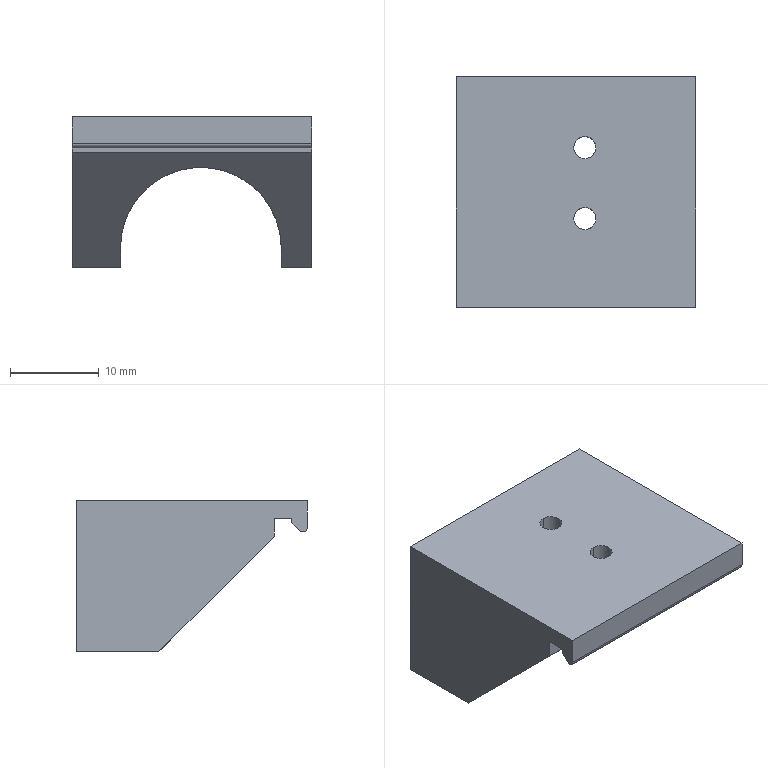NC program | NX | posted with a generic post | part box 27 x 26 x 17 mm
Lines 1 to 1768 of 22937, first 1687 of 1754 lines:
N10 G17 G21 G94 G90
(FLOOR_WALL , TOOL : D10JING)
N12 T09 M6
N14 G54
N16 G17 G0 G90 X-23.5 Y14.997 S9500 M3
N18 G43 Z30. H9
N20 Z3.
N22 G94 G1 Z0. F1250.
N24 X-20.5
N26 X20.5
N28 Y10.664
N30 X-20.5
N32 Y6.331
N34 X20.5
N36 Y1.999
N38 X-20.5
N40 Y-2.334
N42 X20.5
N44 Y-6.667
N46 X-20.5
N48 Y-11.
N50 X20.5
N52 X23.5
N54 Z3.
N56 G0 Z30.
N58 M5
(DRILLING , TOOL : D6A45)
N60 T07 M6
N62 G54
N64 G17 G0 G90 X-1. Y-3. S5000 M3
N66 G43 Z30. H7
N68 G94 G81 G98 Z-1. F250. R3.
N70 Y5.
N72 G80
N74 G0 X-1. Y5. Z30.
N76 M5
(DRILLING_COPY_COPY_COPY_COPY , TOOL : 2.5ZT)
N78 T08 M6
N80 G54
N82 G17 G0 G90 X-1. Y5. S2000 M3
N84 G43 Z30. H8
N86 G94 G83 G98 Z-19.251 F150. Q2. R3.
N88 Y-3.
N90 G80
N92 G0 X-1. Y-3. Z30.
N94 M5
(ZLEVEL_PROFILE , TOOL : D10)
N96 T10 M6
N98 G54
N100 G17 G0 G90 X16.359 Y-17.223 S9500 M3
N102 G43 Z30. H10
N104 Z1.5
N106 G94 G1 X15.398 Y-17.766 Z1.442 F1000.
N108 X14.054 Y-18.1 Z1.37
N110 X-14.054 Z-0.104
N112 X-15.398 Y-17.766 Z-0.176
N114 X-16.604 Y-17.084 Z-0.249
N116 X-17.584 Y-16.104 Z-0.321
N118 X-18.266 Y-14.898 Z-0.394
N120 X-18.6 Y-13.554 Z-0.467
N122 Y-13. Z-0.496
N124 Y13. F2500.
N126 G2 X-13.5 Y18.1 R5.1
N128 G1 X13.5
N130 G2 X18.6 Y13. R5.1
N132 G1 Y-13.
N134 G2 X13.5 Y-18.1 R5.1
N136 G1 X-13.5
N138 G2 X-18.6 Y-13. R5.1
N140 G1 Y12.323 Z-0.938
N142 Y12.706 Z-0.944
N144 X-18.599 Y13.09 Z-0.951
N146 X-18.578 Y13.473 Z-0.958
N148 X-18.528 Y13.853 Z-0.964
N150 X-18.45 Y14.229 Z-0.971
N152 X-18.343 Y14.598 Z-0.978
N154 X-18.21 Y14.957 Z-0.984
N156 X-18.049 Y15.305 Z-0.991
N158 G2 X-13.5 Y18.1 R5.1
N160 G1 X13.5
N162 G2 X18.6 Y13. R5.1
N164 G1 Y-13.
N166 G2 X13.5 Y-18.1 R5.1
N168 G1 X-13.5
N170 G2 X-18.6 Y-13. R5.1
N172 G1 Y12.323 Z-1.433
N174 Y12.706 Z-1.44
N176 X-18.599 Y13.09 Z-1.447
N178 X-18.578 Y13.473 Z-1.453
N180 X-18.528 Y13.853 Z-1.46
N182 X-18.45 Y14.229 Z-1.467
N184 X-18.343 Y14.598 Z-1.473
N186 X-18.21 Y14.957 Z-1.48
N188 X-18.049 Y15.305 Z-1.487
N190 G2 X-13.5 Y18.1 R5.1
N192 G1 X13.5
N194 G2 X18.6 Y13. R5.1
N196 G1 Y-13.
N198 G2 X13.5 Y-18.1 R5.1
N200 G1 X-13.5
N202 G2 X-18.6 Y-13. R5.1
N204 G1 Y12.323 Z-1.929
N206 Y12.706 Z-1.935
N208 X-18.599 Y13.09 Z-1.942
N210 X-18.578 Y13.473 Z-1.949
N212 X-18.528 Y13.853 Z-1.956
N214 X-18.45 Y14.229 Z-1.962
N216 X-18.343 Y14.598 Z-1.969
N218 X-18.21 Y14.957 Z-1.976
N220 X-18.049 Y15.305 Z-1.982
N222 G2 X-13.5 Y18.1 R5.1
N224 G1 X13.5
N226 G2 X18.6 Y13. R5.1
N228 G1 Y-13.
N230 G2 X13.5 Y-18.1 R5.1
N232 G1 X-13.5
N234 G2 X-18.6 Y-13. R5.1
N236 G1 Y12.323 Z-2.424
N238 Y12.706 Z-2.431
N240 X-18.599 Y13.09 Z-2.438
N242 X-18.578 Y13.473 Z-2.444
N244 X-18.528 Y13.853 Z-2.451
N246 X-18.45 Y14.229 Z-2.458
N248 X-18.343 Y14.598 Z-2.465
N250 X-18.21 Y14.957 Z-2.471
N252 X-18.049 Y15.305 Z-2.478
N254 G2 X-13.5 Y18.1 R5.1
N256 G1 X13.5
N258 G2 X18.6 Y13. R5.1
N260 G1 Y-13.
N262 G2 X13.5 Y-18.1 R5.1
N264 G1 X-13.5
N266 G2 X-18.6 Y-13. R5.1
N268 G1 Y12.323 Z-2.92
N270 Y12.706 Z-2.927
N272 X-18.599 Y13.09 Z-2.933
N274 X-18.578 Y13.473 Z-2.94
N276 X-18.528 Y13.853 Z-2.947
N278 X-18.45 Y14.229 Z-2.953
N280 X-18.343 Y14.598 Z-2.96
N282 X-18.21 Y14.957 Z-2.967
N284 X-18.049 Y15.305 Z-2.974
N286 G2 X-13.5 Y18.1 R5.1
N288 G1 X13.5
N290 G2 X18.6 Y13. R5.1
N292 G1 Y-13.
N294 G2 X13.5 Y-18.1 R5.1
N296 G1 X-13.5
N298 G2 X-18.6 Y-13. R5.1
N300 G1 Y12.323 Z-3.416
N302 Y12.706 Z-3.422
N304 X-18.599 Y13.09 Z-3.429
N306 X-18.578 Y13.473 Z-3.436
N308 X-18.528 Y13.853 Z-3.442
N310 X-18.45 Y14.229 Z-3.449
N312 X-18.343 Y14.598 Z-3.456
N314 X-18.21 Y14.957 Z-3.462
N316 X-18.049 Y15.305 Z-3.469
N318 G2 X-13.5 Y18.1 R5.1
N320 G1 X13.5
N322 G2 X18.6 Y13. R5.1
N324 G1 Y-13.
N326 G2 X13.5 Y-18.1 R5.1
N328 G1 X-13.5
N330 G2 X-18.6 Y-13. R5.1
N332 G1 Y12.323 Z-3.911
N334 Y12.706 Z-3.918
N336 X-18.599 Y13.09 Z-3.925
N338 X-18.578 Y13.473 Z-3.931
N340 X-18.528 Y13.853 Z-3.938
N342 X-18.45 Y14.229 Z-3.945
N344 X-18.343 Y14.598 Z-3.951
N346 X-18.21 Y14.957 Z-3.958
N348 X-18.049 Y15.305 Z-3.965
N350 G2 X-13.5 Y18.1 R5.1
N352 G1 X13.5
N354 G2 X18.6 Y13. R5.1
N356 G1 Y-13.
N358 G2 X13.5 Y-18.1 R5.1
N360 G1 X-13.5
N362 G2 X-18.6 Y-13. R5.1
N364 G1 Y12.323 Z-4.407
N366 Y12.706 Z-4.413
N368 X-18.599 Y13.09 Z-4.42
N370 X-18.578 Y13.473 Z-4.427
N372 X-18.528 Y13.853 Z-4.434
N374 X-18.45 Y14.229 Z-4.44
N376 X-18.343 Y14.598 Z-4.447
N378 X-18.21 Y14.957 Z-4.454
N380 X-18.049 Y15.305 Z-4.46
N382 G2 X-13.5 Y18.1 R5.1
N384 G1 X13.5
N386 G2 X18.6 Y13. R5.1
N388 G1 Y-13.
N390 G2 X13.5 Y-18.1 R5.1
N392 G1 X-13.5
N394 G2 X-18.6 Y-13. R5.1
N396 G1 Y12.323 Z-4.902
N398 Y12.706 Z-4.909
N400 X-18.599 Y13.09 Z-4.916
N402 X-18.578 Y13.473 Z-4.922
N404 X-18.528 Y13.853 Z-4.929
N406 X-18.45 Y14.229 Z-4.936
N408 X-18.343 Y14.598 Z-4.942
N410 X-18.21 Y14.957 Z-4.949
N412 X-18.049 Y15.305 Z-4.956
N414 G2 X-13.5 Y18.1 R5.1
N416 G1 X13.5
N418 G2 X18.6 Y13. R5.1
N420 G1 Y-13.
N422 G2 X13.5 Y-18.1 R5.1
N424 G1 X-13.5
N426 G2 X-18.6 Y-13. R5.1
N428 G1 Y12.323 Z-5.398
N430 Y12.706 Z-5.405
N432 X-18.599 Y13.09 Z-5.411
N434 X-18.578 Y13.473 Z-5.418
N436 X-18.528 Y13.853 Z-5.425
N438 X-18.45 Y14.229 Z-5.431
N440 X-18.343 Y14.598 Z-5.438
N442 X-18.21 Y14.957 Z-5.445
N444 X-18.049 Y15.305 Z-5.451
N446 G2 X-13.5 Y18.1 R5.1
N448 G1 X13.5
N450 G2 X18.6 Y13. R5.1
N452 G1 Y-13.
N454 G2 X13.5 Y-18.1 R5.1
N456 G1 X-13.5
N458 G2 X-18.6 Y-13. R5.1
N460 G1 Y12.323 Z-5.893
N462 Y12.706 Z-5.9
N464 X-18.599 Y13.09 Z-5.907
N466 X-18.578 Y13.473 Z-5.914
N468 X-18.528 Y13.853 Z-5.92
N470 X-18.45 Y14.229 Z-5.927
N472 X-18.343 Y14.598 Z-5.934
N474 X-18.21 Y14.957 Z-5.94
N476 X-18.049 Y15.305 Z-5.947
N478 G2 X-13.5 Y18.1 R5.1
N480 G1 X13.5
N482 G2 X18.6 Y13. R5.1
N484 G1 Y-13.
N486 G2 X13.5 Y-18.1 R5.1
N488 G1 X-13.5
N490 G2 X-18.6 Y-13. R5.1
N492 G1 Y12.323 Z-6.389
N494 Y12.706 Z-6.396
N496 X-18.599 Y13.09 Z-6.402
N498 X-18.578 Y13.473 Z-6.409
N500 X-18.528 Y13.853 Z-6.416
N502 X-18.45 Y14.229 Z-6.423
N504 X-18.343 Y14.598 Z-6.429
N506 X-18.21 Y14.957 Z-6.436
N508 X-18.049 Y15.305 Z-6.443
N510 G2 X-13.5 Y18.1 R5.1
N512 G1 X13.5
N514 G2 X18.6 Y13. R5.1
N516 G1 Y-13.
N518 G2 X13.5 Y-18.1 R5.1
N520 G1 X-13.5
N522 G2 X-18.6 Y-13. R5.1
N524 G1 Y12.323 Z-6.885
N526 Y12.706 Z-6.891
N528 X-18.599 Y13.09 Z-6.898
N530 X-18.578 Y13.473 Z-6.905
N532 X-18.528 Y13.853 Z-6.911
N534 X-18.45 Y14.229 Z-6.918
N536 X-18.343 Y14.598 Z-6.925
N538 X-18.21 Y14.957 Z-6.932
N540 X-18.049 Y15.305 Z-6.938
N542 G2 X-13.5 Y18.1 R5.1
N544 G1 X13.5
N546 G2 X18.6 Y13. R5.1
N548 G1 Y-13.
N550 G2 X13.5 Y-18.1 R5.1
N552 G1 X-13.5
N554 G2 X-18.6 Y-13. R5.1
N556 G1 Y12.323 Z-7.38
N558 Y12.706 Z-7.387
N560 X-18.599 Y13.09 Z-7.394
N562 X-18.578 Y13.473 Z-7.4
N564 X-18.528 Y13.853 Z-7.407
N566 X-18.45 Y14.229 Z-7.414
N568 X-18.343 Y14.598 Z-7.42
N570 X-18.21 Y14.957 Z-7.427
N572 X-18.049 Y15.305 Z-7.434
N574 G2 X-13.5 Y18.1 R5.1
N576 G1 X13.5
N578 G2 X18.6 Y13. R5.1
N580 G1 Y-13.
N582 G2 X13.5 Y-18.1 R5.1
N584 G1 X-13.5
N586 G2 X-18.6 Y-13. R5.1
N588 G1 Y12.323 Z-7.876
N590 Y12.706 Z-7.883
N592 X-18.599 Y13.09 Z-7.889
N594 X-18.578 Y13.473 Z-7.896
N596 X-18.528 Y13.853 Z-7.903
N598 X-18.45 Y14.229 Z-7.909
N600 X-18.343 Y14.598 Z-7.916
N602 X-18.21 Y14.957 Z-7.923
N604 X-18.049 Y15.305 Z-7.929
N606 G2 X-13.5 Y18.1 R5.1
N608 G1 X13.5
N610 G2 X18.6 Y13. R5.1
N612 G1 Y-13.
N614 G2 X13.5 Y-18.1 R5.1
N616 G1 X-13.5
N618 G2 X-18.6 Y-13. R5.1
N620 G1 Y12.323 Z-8.371
N622 Y12.706 Z-8.378
N624 X-18.599 Y13.09 Z-8.385
N626 X-18.578 Y13.473 Z-8.392
N628 X-18.528 Y13.853 Z-8.398
N630 X-18.45 Y14.229 Z-8.405
N632 X-18.343 Y14.598 Z-8.412
N634 X-18.21 Y14.957 Z-8.418
N636 X-18.049 Y15.305 Z-8.425
N638 G2 X-13.5 Y18.1 R5.1
N640 G1 X13.5
N642 G2 X18.6 Y13. R5.1
N644 G1 Y-13.
N646 G2 X13.5 Y-18.1 R5.1
N648 G1 X-13.5
N650 G2 X-18.6 Y-13. R5.1
N652 G1 Y12.323 Z-8.867
N654 Y12.706 Z-8.874
N656 X-18.599 Y13.09 Z-8.88
N658 X-18.578 Y13.473 Z-8.887
N660 X-18.528 Y13.853 Z-8.894
N662 X-18.45 Y14.229 Z-8.9
N664 X-18.343 Y14.598 Z-8.907
N666 X-18.21 Y14.957 Z-8.914
N668 X-18.049 Y15.305 Z-8.921
N670 G2 X-13.5 Y18.1 R5.1
N672 G1 X13.5
N674 G2 X18.6 Y13. R5.1
N676 G1 Y-13.
N678 G2 X13.5 Y-18.1 R5.1
N680 G1 X-13.5
N682 G2 X-18.6 Y-13. R5.1
N684 G1 Y12.323 Z-9.363
N686 Y12.706 Z-9.369
N688 X-18.599 Y13.09 Z-9.376
N690 X-18.578 Y13.473 Z-9.383
N692 X-18.528 Y13.853 Z-9.389
N694 X-18.45 Y14.229 Z-9.396
N696 X-18.343 Y14.598 Z-9.403
N698 X-18.21 Y14.957 Z-9.409
N700 X-18.049 Y15.305 Z-9.416
N702 G2 X-13.5 Y18.1 R5.1
N704 G1 X13.5
N706 G2 X18.6 Y13. R5.1
N708 G1 Y-13.
N710 G2 X13.5 Y-18.1 R5.1
N712 G1 X-13.5
N714 G2 X-18.6 Y-13. R5.1
N716 G1 Y12.323 Z-9.858
N718 Y12.706 Z-9.865
N720 X-18.599 Y13.09 Z-9.872
N722 X-18.578 Y13.473 Z-9.878
N724 X-18.528 Y13.853 Z-9.885
N726 X-18.45 Y14.229 Z-9.892
N728 X-18.343 Y14.598 Z-9.898
N730 X-18.21 Y14.957 Z-9.905
N732 X-18.049 Y15.305 Z-9.912
N734 G2 X-13.5 Y18.1 R5.1
N736 G1 X13.5
N738 G2 X18.6 Y13. R5.1
N740 G1 Y-13.
N742 G2 X13.5 Y-18.1 R5.1
N744 G1 X-13.5
N746 G2 X-18.6 Y-13. R5.1
N748 G1 Y12.323 Z-10.354
N750 Y12.706 Z-10.36
N752 X-18.599 Y13.09 Z-10.367
N754 X-18.578 Y13.473 Z-10.374
N756 X-18.528 Y13.853 Z-10.381
N758 X-18.45 Y14.229 Z-10.387
N760 X-18.343 Y14.598 Z-10.394
N762 X-18.21 Y14.957 Z-10.401
N764 X-18.049 Y15.305 Z-10.407
N766 G2 X-13.5 Y18.1 R5.1
N768 G1 X13.5
N770 G2 X18.6 Y13. R5.1
N772 G1 Y-13.
N774 G2 X13.5 Y-18.1 R5.1
N776 G1 X-13.5
N778 G2 X-18.6 Y-13. R5.1
N780 G1 Y12.323 Z-10.849
N782 Y12.706 Z-10.856
N784 X-18.599 Y13.09 Z-10.863
N786 X-18.578 Y13.473 Z-10.869
N788 X-18.528 Y13.853 Z-10.876
N790 X-18.45 Y14.229 Z-10.883
N792 X-18.343 Y14.598 Z-10.89
N794 X-18.21 Y14.957 Z-10.896
N796 X-18.049 Y15.305 Z-10.903
N798 G2 X-13.5 Y18.1 R5.1
N800 G1 X13.5
N802 G2 X18.6 Y13. R5.1
N804 G1 Y-13.
N806 G2 X13.5 Y-18.1 R5.1
N808 G1 X-13.5
N810 G2 X-18.6 Y-13. R5.1
N812 G1 Y12.323 Z-11.345
N814 Y12.706 Z-11.352
N816 X-18.599 Y13.09 Z-11.358
N818 X-18.578 Y13.473 Z-11.365
N820 X-18.528 Y13.853 Z-11.372
N822 X-18.45 Y14.229 Z-11.378
N824 X-18.343 Y14.598 Z-11.385
N826 X-18.21 Y14.957 Z-11.392
N828 X-18.049 Y15.305 Z-11.399
N830 G2 X-13.5 Y18.1 R5.1
N832 G1 X13.5
N834 G2 X18.6 Y13. R5.1
N836 G1 Y-13.
N838 G2 X13.5 Y-18.1 R5.1
N840 G1 X-13.5
N842 G2 X-18.6 Y-13. R5.1
N844 G1 Y12.323 Z-11.841
N846 Y12.706 Z-11.847
N848 X-18.599 Y13.09 Z-11.854
N850 X-18.578 Y13.473 Z-11.861
N852 X-18.528 Y13.853 Z-11.867
N854 X-18.45 Y14.229 Z-11.874
N856 X-18.343 Y14.598 Z-11.881
N858 X-18.21 Y14.957 Z-11.887
N860 X-18.049 Y15.305 Z-11.894
N862 G2 X-13.5 Y18.1 R5.1
N864 G1 X13.5
N866 G2 X18.6 Y13. R5.1
N868 G1 Y-13.
N870 G2 X13.5 Y-18.1 R5.1
N872 G1 X-13.5
N874 G2 X-18.6 Y-13. R5.1
N876 G1 Y12.323 Z-12.336
N878 Y12.706 Z-12.343
N880 X-18.599 Y13.09 Z-12.35
N882 X-18.578 Y13.473 Z-12.356
N884 X-18.528 Y13.853 Z-12.363
N886 X-18.45 Y14.229 Z-12.37
N888 X-18.343 Y14.598 Z-12.376
N890 X-18.21 Y14.957 Z-12.383
N892 X-18.049 Y15.305 Z-12.39
N894 G2 X-13.5 Y18.1 R5.1
N896 G1 X13.5
N898 G2 X18.6 Y13. R5.1
N900 G1 Y-13.
N902 G2 X13.5 Y-18.1 R5.1
N904 G1 X-13.5
N906 G2 X-18.6 Y-13. R5.1
N908 G1 Y12.323 Z-12.832
N910 Y12.706 Z-12.838
N912 X-18.599 Y13.09 Z-12.845
N914 X-18.578 Y13.473 Z-12.852
N916 X-18.528 Y13.853 Z-12.859
N918 X-18.45 Y14.229 Z-12.865
N920 X-18.343 Y14.598 Z-12.872
N922 X-18.21 Y14.957 Z-12.879
N924 X-18.049 Y15.305 Z-12.885
N926 G2 X-13.5 Y18.1 R5.1
N928 G1 X13.5
N930 G2 X18.6 Y13. R5.1
N932 G1 Y-13.
N934 G2 X13.5 Y-18.1 R5.1
N936 G1 X-13.5
N938 G2 X-18.6 Y-13. R5.1
N940 G1 Y12.323 Z-13.327
N942 Y12.706 Z-13.334
N944 X-18.599 Y13.09 Z-13.341
N946 X-18.578 Y13.473 Z-13.347
N948 X-18.528 Y13.853 Z-13.354
N950 X-18.45 Y14.229 Z-13.361
N952 X-18.343 Y14.598 Z-13.367
N954 X-18.21 Y14.957 Z-13.374
N956 X-18.049 Y15.305 Z-13.381
N958 G2 X-13.5 Y18.1 R5.1
N960 G1 X13.5
N962 G2 X18.6 Y13. R5.1
N964 G1 Y-13.
N966 G2 X13.5 Y-18.1 R5.1
N968 G1 X-13.5
N970 G2 X-18.6 Y-13. R5.1
N972 G1 Y12.323 Z-13.823
N974 Y12.706 Z-13.83
N976 X-18.599 Y13.09 Z-13.836
N978 X-18.578 Y13.473 Z-13.843
N980 X-18.528 Y13.853 Z-13.85
N982 X-18.45 Y14.229 Z-13.856
N984 X-18.343 Y14.598 Z-13.863
N986 X-18.21 Y14.957 Z-13.87
N988 X-18.049 Y15.305 Z-13.876
N990 G2 X-13.5 Y18.1 R5.1
N992 G1 X13.5
N994 G2 X18.6 Y13. R5.1
N996 G1 Y-13.
N998 G2 X13.5 Y-18.1 R5.1
N1000 G1 X-13.5
N1002 G2 X-18.6 Y-13. R5.1
N1004 G1 Y12.323 Z-14.318
N1006 Y12.706 Z-14.325
N1008 X-18.599 Y13.09 Z-14.332
N1010 X-18.578 Y13.473 Z-14.339
N1012 X-18.528 Y13.853 Z-14.345
N1014 X-18.45 Y14.229 Z-14.352
N1016 X-18.343 Y14.598 Z-14.359
N1018 X-18.21 Y14.957 Z-14.365
N1020 X-18.049 Y15.305 Z-14.372
N1022 G2 X-13.5 Y18.1 R5.1
N1024 G1 X13.5
N1026 G2 X18.6 Y13. R5.1
N1028 G1 Y-13.
N1030 G2 X13.5 Y-18.1 R5.1
N1032 G1 X-13.5
N1034 G2 X-18.6 Y-13. R5.1
N1036 G1 Y12.323 Z-14.814
N1038 Y12.706 Z-14.821
N1040 X-18.599 Y13.09 Z-14.827
N1042 X-18.578 Y13.473 Z-14.834
N1044 X-18.528 Y13.853 Z-14.841
N1046 X-18.45 Y14.229 Z-14.848
N1048 X-18.343 Y14.598 Z-14.854
N1050 X-18.21 Y14.957 Z-14.861
N1052 X-18.049 Y15.305 Z-14.868
N1054 G2 X-13.5 Y18.1 R5.1
N1056 G1 X13.5
N1058 G2 X18.6 Y13. R5.1
N1060 G1 Y-13.
N1062 G2 X13.5 Y-18.1 R5.1
N1064 G1 X-13.5
N1066 G2 X-18.6 Y-13. R5.1
N1068 G1 Y12.323 Z-15.31
N1070 Y12.706 Z-15.316
N1072 X-18.599 Y13.09 Z-15.323
N1074 X-18.578 Y13.473 Z-15.33
N1076 X-18.528 Y13.853 Z-15.336
N1078 X-18.45 Y14.229 Z-15.343
N1080 X-18.343 Y14.598 Z-15.35
N1082 X-18.21 Y14.957 Z-15.357
N1084 X-18.049 Y15.305 Z-15.363
N1086 G2 X-13.5 Y18.1 R5.1
N1088 G1 X13.5
N1090 G2 X18.6 Y13. R5.1
N1092 G1 Y-13.
N1094 G2 X13.5 Y-18.1 R5.1
N1096 G1 X-13.5
N1098 G2 X-18.6 Y-13. R5.1
N1100 G1 Y12.323 Z-15.805
N1102 Y12.706 Z-15.812
N1104 X-18.599 Y13.09 Z-15.819
N1106 X-18.578 Y13.473 Z-15.825
N1108 X-18.528 Y13.853 Z-15.832
N1110 X-18.45 Y14.229 Z-15.839
N1112 X-18.343 Y14.598 Z-15.845
N1114 X-18.21 Y14.957 Z-15.852
N1116 X-18.049 Y15.305 Z-15.859
N1118 G2 X-13.5 Y18.1 R5.1
N1120 G1 X13.5
N1122 G2 X18.6 Y13. R5.1
N1124 G1 Y-13.
N1126 G2 X13.5 Y-18.1 R5.1
N1128 G1 X-13.5
N1130 G2 X-18.6 Y-13. R5.1
N1132 G1 Y12.323 Z-16.301
N1134 Y12.706 Z-16.308
N1136 X-18.599 Y13.09 Z-16.314
N1138 X-18.578 Y13.473 Z-16.321
N1140 X-18.528 Y13.853 Z-16.328
N1142 X-18.45 Y14.229 Z-16.334
N1144 X-18.343 Y14.598 Z-16.341
N1146 X-18.21 Y14.957 Z-16.348
N1148 X-18.049 Y15.305 Z-16.354
N1150 G2 X-13.5 Y18.1 R5.1
N1152 G1 X13.5
N1154 G2 X18.6 Y13. R5.1
N1156 G1 Y-13.
N1158 G2 X13.5 Y-18.1 R5.1
N1160 G1 X-13.5
N1162 G2 X-18.6 Y-13. R5.1
N1164 G1 Y12.323 Z-16.796
N1166 Y12.706 Z-16.803
N1168 X-18.599 Y13.09 Z-16.81
N1170 X-18.578 Y13.473 Z-16.817
N1172 X-18.528 Y13.853 Z-16.823
N1174 X-18.45 Y14.229 Z-16.83
N1176 X-18.343 Y14.598 Z-16.837
N1178 X-18.21 Y14.957 Z-16.843
N1180 X-18.049 Y15.305 Z-16.85
N1182 G2 X-13.5 Y18.1 R5.1
N1184 G1 X13.5
N1186 G2 X18.6 Y13. R5.1
N1188 G1 Y-13.
N1190 G2 X13.5 Y-18.1 R5.1
N1192 G1 X-13.5
N1194 G2 X-18.6 Y-13. R5.1
N1196 G1 Y13.
N1198 G2 X-18.049 Y15.305 R5.1
N1200 G1 Z-15.35
N1202 G0 Z30.
(CAVITY_MILL , TOOL : D10)
N1204 X3.912 Y-22.799
N1206 Z1.003
N1208 G1 Z-0.497 F1000.
N1210 X-0.129 Y-15.799
N1212 G3 X-0.995 Y-15.299 R1.
N1214 G1 Y-8.299
N1216 X4.307 F3000.
N1218 X9.996 Y-8.642
N1220 X4.307 Y-8.299
N1222 G2 X-0.997 Y-4.801 R12.132
N1224 X-6.298 Y-8.299 R12.121
N1226 G1 X-0.995
N1228 Y-15.299
N1230 X15.502
N1232 G3 X15.799 Y-15.002 R0.297
N1234 G1 Y-2.88
N1236 G3 X18.5 Y-0.945 R6.526
N1238 G1 Y2.21
N1240 G2 X13.5 Y-1.908 R5.126
N1242 G1 X8.07
N1244 G2 X2.97 Y3.233 R5.132
N1246 G1 Y13.
N1248 G2 X7.065 Y18. R5.1
N1250 G1 X3.917
N1252 G3 X1.99 Y15.299 R6.5
N1254 G1 X-3.99
N1256 G3 X-5.917 Y18. R6.5
N1258 G1 X-9.065
N1260 G2 X-4.971 Y13.091 R5.1
N1262 G1 X-4.97 Y13.
N1264 Y3.233
N1266 G2 X-10.07 Y-1.908 R5.121
N1268 G1 X-13.5
N1270 G2 X-18.5 Y2.21 R5.126
N1272 G1 Y-0.945
N1274 G3 X-15.799 Y-2.88 R6.526
N1276 G1 Y-15.002
N1278 G3 X-15.502 Y-15.299 R0.297
N1280 G1 X-0.995
N1282 G2 X-0.129 Y-15.799 R1.
N1284 G1 X3.912 Y-22.799
N1286 Z1.003
N1288 G0 X3.91 Z0.507
N1290 G1 Z-0.993 F1000.
N1292 X-0.131 Y-15.799
N1294 G3 X-0.997 Y-15.299 R1.
N1296 G1 Y-8.299
N1298 X3.039 F3000.
N1300 X9.365 Y-8.88
N1302 X3.039 Y-8.299
N1304 G2 X-0.998 Y-5.299 R12.128
N1306 X-5.033 Y-8.299 R12.121
N1308 G1 X-10.357 Y-8.944
N1310 X-5.033 Y-8.299
N1312 X-0.997
N1314 Y-15.299
N1316 X15.502
N1318 G3 X15.799 Y-15.002 R0.297
N1320 G1 Y-3.378
N1322 G3 X18.5 Y-1.445 R6.521
N1324 G1 Y1.709
N1326 G2 X13.5 Y-2.405 R5.121
N1328 G1 X8.049
N1330 G2 X2.97 Y2.737 R5.128
N1332 G1 Y13.
N1334 G2 X7.065 Y18. R5.1
N1336 G1 X3.917
N1338 G3 X1.99 Y15.299 R6.5
N1340 G1 X-3.99
N1342 G3 X-5.917 Y18. R6.5
N1344 G1 X-9.065
N1346 G2 X-4.971 Y13.091 R5.1
N1348 G1 X-4.97 Y13.
N1350 Y2.737
N1352 G2 X-10.07 Y-2.405 R5.121
N1354 G1 X-13.5
N1356 G2 X-18.5 Y1.709 R5.121
N1358 G1 Y-1.445
N1360 G3 X-15.799 Y-3.378 R6.521
N1362 G1 Y-15.002
N1364 G3 X-15.502 Y-15.299 R0.297
N1366 G1 X-0.997
N1368 G2 X-0.131 Y-15.799 R1.
N1370 G1 X3.91 Y-22.799
N1372 Z0.507
N1374 G0 Z0.01
N1376 G1 Z-1.49 F1000.
N1378 X-0.132 Y-15.799
N1380 G3 X-0.998 Y-15.299 R1.
N1382 G1 Y-8.299
N1384 X2.072 F3000.
N1386 X8.873 Y-9.119
N1388 X2.072 Y-8.299
N1390 G2 X-0.998 Y-5.796 R12.127
N1392 X-4.068 Y-8.299 R12.121
N1394 G1 X-9.87 Y-9.138
N1396 X-4.068 Y-8.299
N1398 X-0.998
N1400 Y-15.299
N1402 X15.502
N1404 G3 X15.799 Y-15.002 R0.297
N1406 G1 Y-3.875
N1408 G3 X18.5 Y-1.942 R6.521
N1410 G1 Y1.212
N1412 G2 X13.5 Y-2.901 R5.121
N1414 G1 X8.07
N1416 G2 X2.97 Y2.24 R5.127
N1418 G1 Y13.
N1420 G2 X7.065 Y18. R5.1
N1422 G1 X3.917
N1424 G3 X1.99 Y15.299 R6.5
N1426 G1 X-3.99
N1428 G3 X-5.917 Y18. R6.5
N1430 G1 X-9.065
N1432 G2 X-4.971 Y13.09 R5.1
N1434 G1 X-4.97 Y13.
N1436 Y2.24
N1438 G2 X-10.07 Y-2.901 R5.121
N1440 G1 X-13.5
N1442 G2 X-18.5 Y1.212 R5.121
N1444 G1 Y-1.942
N1446 G3 X-15.799 Y-3.875 R6.521
N1448 G1 Y-15.002
N1450 G3 X-15.502 Y-15.299 R0.297
N1452 G1 X-0.998
N1454 G2 X-0.132 Y-15.799 R1.
N1456 G1 X3.91 Y-22.799
N1458 Z0.01
N1460 G0 X3.907 Z-0.487
N1462 G1 Z-1.987 F1000.
N1464 X-0.134 Y-15.799
N1466 G3 X-1. Y-15.299 R1.
N1468 G1 Y-8.299
N1470 X1.274 F3000.
N1472 X8.444 Y-9.352
N1474 X1.274 Y-8.299
N1476 G2 X-1. Y-6.294 R12.121
N1478 X-3.274 Y-8.299 R12.121
N1480 G1 X-9.448 Y-9.354
N1482 X-3.274 Y-8.299
N1484 X-1.
N1486 Y-15.299
N1488 X15.502
N1490 G3 X15.799 Y-15.002 R0.297
N1492 G1 Y-4.37
N1494 G3 X18.5 Y-2.436 R6.524
N1496 G1 Y0.718
N1498 G2 X13.5 Y-3.398 R5.124
N1500 G1 X8.07
N1502 G2 X2.97 Y1.743 R5.121
N1504 G1 Y13.
N1506 G2 X7.065 Y18. R5.1
N1508 G1 X3.917
N1510 G3 X1.99 Y15.299 R6.5
N1512 G1 X-3.99
N1514 G3 X-5.917 Y18. R6.5
N1516 G1 X-9.065
N1518 G2 X-4.971 Y13.091 R5.1
N1520 G1 X-4.97 Y13.
N1522 Y1.743
N1524 G2 X-10.07 Y-3.398 R5.121
N1526 G1 X-13.5
N1528 G2 X-18.5 Y0.725 R5.131
N1530 G1 Y-2.432
N1532 G3 X-15.799 Y-4.368 R6.531
N1534 G1 Y-15.002
N1536 G3 X-15.502 Y-15.299 R0.297
N1538 G1 X-1.
N1540 G2 X-0.134 Y-15.799 R1.
N1542 G1 X3.907 Y-22.799
N1544 Z-0.487
N1546 G0 Z-0.983
N1548 G1 Z-2.483 F1000.
N1550 X-0.134 Y-15.799
N1552 G3 X-1. Y-15.299 R1.
N1554 G1 Y-8.299
N1556 X0.587 F3000.
N1558 X8.033 Y-9.578
N1560 X0.587 Y-8.299
N1562 G2 X-1. Y-6.8 R12.114
N1564 X-2.587 Y-8.299 R12.114
N1566 G1 X-9.049 Y-9.568
N1568 X-2.587 Y-8.299
N1570 X-1.
N1572 Y-15.299
N1574 X15.502
N1576 G3 X15.799 Y-15.002 R0.297
N1578 G1 Y-4.868
N1580 G3 X18.5 Y-2.935 R6.521
N1582 G1 Y0.219
N1584 G2 X13.5 Y-3.895 R5.121
N1586 G1 X8.056
N1588 G2 X2.966 Y1.244 R5.114
N1590 G1 Y12.965
N1592 G2 X5.955 Y17.641 R5.041
N1594 X7.065 Y18. R5.1
N1596 G1 X3.902
N1598 G3 X1.976 Y15.299 R6.441
N1600 G1 X-3.987
N1602 G3 X-5.914 Y18. R6.502
N1604 G1 X-9.063
N1606 G2 X-4.966 Y13. R5.102
N1608 G1 Y1.244
N1610 G2 X-10.056 Y-3.895 R5.114
N1612 G1 X-13.5
N1614 G2 X-18.5 Y0.219 R5.121
N1616 G1 Y-2.935
N1618 G3 X-15.799 Y-4.868 R6.521
N1620 G1 Y-15.002
N1622 G3 X-15.502 Y-15.299 R0.297
N1624 G1 X-1.
N1626 G2 X-0.134 Y-15.799 R1.
N1628 G1 X3.907 Y-22.799
N1630 Z-0.983
N1632 G0 X3.909 Z-1.48
N1634 G1 Z-2.98 F1000.
N1636 X-0.133 Y-15.799
N1638 G3 X-0.999 Y-15.299 R1.
N1640 G1 Y-8.299
N1642 X-0.036 F3000.
N1644 X7.574 Y-9.796
N1646 X-0.036 Y-8.299
N1648 G2 X-0.999 Y-7.333 R12.111
N1650 X-1.962 Y-8.299 R12.11
N1652 G1 X-8.619 Y-9.776
N1654 X-1.962 Y-8.299
N1656 X-0.999
N1658 Y-15.299
N1660 X15.502
N1662 G3 X15.799 Y-15.002 R0.297
N1664 G1 Y-5.365
N1666 G3 X18.5 Y-3.432 R6.521
N1668 G1 Y-0.278
N1670 G2 X13.5 Y-4.391 R5.121
N1672 G1 X8.026
N1674 G2 X2.936 Y0.741 R5.111
N1676 G1 Y12.934
N1678 G2 X6.997 Y18. R5.066
N1680 G1 X3.86
N1682 G3 X1.945 Y15.299 R6.466
N1684 G1 X-3.946
N1686 G3 X-5.862 Y18. R6.469
N1688 G1 X-9.001
N1690 G2 X-4.936 Y12.975 R5.069
N1692 G1 Y1.156
N1694 X-4.934 Y0.741
N1696 G2 X-10.026 Y-4.391 R5.11
N1698 G1 X-13.5
N1700 G2 X-18.5 Y-0.278 R5.121
N1702 G1 Y-3.432
N1704 G3 X-15.799 Y-5.365 R6.521
N1706 G1 Y-15.002
N1708 G3 X-15.502 Y-15.299 R0.297
N1710 G1 X-0.999
N1712 G2 X-0.133 Y-15.799 R1.
N1714 G1 X3.909 Y-22.799
N1716 Z-1.48
N1718 G0 Z-1.977
N1720 G1 Z-3.477 F1000.
N1722 X-0.132 Y-15.799
N1724 G3 X-0.998 Y-15.299 R1.
N1726 G1 Y-8.299
N1728 X-0.617 F3000.
N1730 X6.87 Y-9.993
N1732 X-0.617 Y-8.299
N1734 G2 X-0.998 Y-7.896 R12.113
N1736 X-1.38 Y-8.299 R12.108
N1738 G1 X-8.023 Y-9.964
N1740 X-1.38 Y-8.299
N1742 X-0.998
N1744 Y-15.299
N1746 X15.502
N1748 G3 X15.799 Y-15.002 R0.297
N1750 G1 Y-5.861
N1752 G3 X18.5 Y-3.928 R6.521
N1754 G1 Y-0.775
N1756 G2 X13.5 Y-4.888 R5.121
N1758 G1 X7.967
N1760 G2 X2.879 Y0.385 R5.113
N1762 G1 Y12.959
N1764 G2 X6.933 Y18. R5.065
N1766 G1 X3.8
N1768 G3 X1.887 Y15.299 R6.465
N1770 G1 X-3.889
N1772 G3 X-5.798 Y18. R6.453
N1774 G1 X-8.927
N1776 G2 X-4.942 Y13.817 R5.053
N1778 X-4.879 Y13.523 R0.711
N1780 G1 Y0.385
N1782 G2 X-9.967 Y-4.888 R5.108
N1784 G1 X-13.5
N1786 G2 X-18.5 Y-0.775 R5.121
N1788 G1 Y-3.928
N1790 G3 X-15.799 Y-5.861 R6.521
N1792 G1 Y-15.002
N1794 G3 X-15.502 Y-15.299 R0.297
N1796 G1 X-0.998
N1798 G2 X-0.132 Y-15.799 R1.
N1800 G1 X3.909 Y-22.799
N1802 Z-1.977
N1804 G0 X4.907 Z-2.473
N1806 G1 Z-3.973 F1000.
N1808 X0.866 Y-15.799
N1810 G3 X0. Y-15.299 R1.
N1812 G1 Y-10.799
N1814 X11.299 F3000.
N1816 Y-9.885
N1818 X7.871
N1820 G2 X-0.998 Y-3.895 R9.574
N1822 X-9.864 Y-9.885 R9.602
N1824 G1 X-11.299
N1826 Y-10.799
N1828 X0.
N1830 Y-15.299
N1832 X15.502
N1834 G3 X15.799 Y-15.002 R0.297
N1836 G1 Y-6.358
N1838 G3 X18.5 Y-4.425 R6.521
N1840 G1 Y-1.271
N1842 G2 X13.5 Y-5.385 R5.121
N1844 G1 X7.874
N1846 G2 X2.825 Y-0.749 R5.074
N1848 X2.793 Y-0.017 R8.476
N1850 G1 Y12.924
N1852 X2.77 Y12.985
N1854 G2 X6.845 Y18. R5.079
N1856 G1 X3.703
N1858 G3 X1.784 Y15.299 R6.479
N1860 G1 X-3.783
N1862 G3 X-5.712 Y18. R6.51
N1864 G1 X-8.862
N1866 G2 X-4.783 Y13.485 R5.11
N1868 G1 X-4.77 Y12.992
N1870 X-4.793 Y12.933
N1872 Y-0.262
N1874 G2 X-9.874 Y-5.385 R5.102
N1876 G1 X-13.5
N1878 G2 X-18.5 Y-1.271 R5.121
N1880 G1 Y-4.425
N1882 G3 X-15.799 Y-6.358 R6.521
N1884 G1 Y-15.002
N1886 G3 X-15.502 Y-15.299 R0.297
N1888 G1 X0.
N1890 G2 X0.866 Y-15.799 R1.
N1892 G1 X4.907 Y-22.799
N1894 Z-2.473
N1896 G0 Z-2.97
N1898 G1 Z-4.47 F1000.
N1900 X0.866 Y-15.799
N1902 G3 X0. Y-15.299 R1.
N1904 G1 Y-10.799
N1906 X11.299 F3000.
N1908 Y-10.381
N1910 X7.748
N1912 G2 X-1. Y-4.67 R9.598
N1914 X-9.748 Y-10.381 R9.598
N1916 G1 X-11.299
N1918 Y-10.799
N1920 X0.
N1922 Y-15.299
N1924 X15.503
N1926 G3 X15.799 Y-15.003 R0.297
N1928 G1 Y-6.855
N1930 G3 X18.5 Y-4.922 R6.521
N1932 G1 Y-1.768
N1934 G2 X13.5 Y-5.881 R5.121
N1936 G1 X7.756
N1938 G2 X2.678 Y-0.764 R5.098
N1940 G1 Y12.915
N1942 X2.65 Y13.007
N1944 G2 X6.738 Y18. R5.093
N1946 G1 X3.592
N1948 G3 X1.668 Y15.299 R6.493
N1950 G1 X-3.671
N1952 G3 X-5.597 Y18. R6.499
N1954 G1 X-8.746
N1956 G2 X-4.651 Y12.982 R5.099
N1958 G1 X-4.678 Y12.923
N1960 Y-0.764
N1962 G2 X-9.756 Y-5.881 R5.098
N1964 G1 X-11.299
N1966 X-13.546
N1968 G2 X-18.5 Y-1.768 R5.121
N1970 G1 Y-4.922
N1972 G3 X-15.799 Y-6.855 R6.521
N1974 G1 Y-15.003
N1976 G3 X-15.503 Y-15.299 R0.297
N1978 G1 X0.
N1980 G2 X0.866 Y-15.799 R1.
N1982 G1 X4.907 Y-22.799
N1984 Z-2.97
N1986 G0 X3.898 Z-3.467
N1988 G1 Z-4.967 F1000.
N1990 X-0.143 Y-15.799
N1992 G3 X-1.009 Y-15.299 R1.
N1994 G1 Y-10.799
N1996 X6.402 F3000.
N1998 G2 X-1.004 Y-5.473 R9.596
N2000 X-8.421 Y-10.799 R9.616
N2002 G1 X-1.009
N2004 Y-15.299
N2006 X15.503
N2008 G3 X15.799 Y-15.003 R0.297
N2010 G1 Y-7.351
N2012 G3 X18.5 Y-5.418 R6.521
N2014 G1 Y-2.265
N2016 G2 X13.5 Y-6.378 R5.121
N2018 G1 X7.613
N2020 G2 X2.533 Y-1.268 R5.096
N2022 G1 Y13.
N2024 X2.509 Y13.485
N2026 X2.661 Y14.165
N2028 G2 X4.949 Y17.337 R4.8
N2030 X6.601 Y18. R4.964
N2032 G1 X3.452
N2034 G3 X1.531 Y15.299 R6.2
N2036 G1 X-3.54
N2038 G3 X-5.453 Y18. R6.461
N2040 G1 X-8.591
N2042 G2 X-4.533 Y12.942 R5.061
N2044 G1 Y-1.268
N2046 G2 X-9.613 Y-6.378 R5.116
N2048 G1 X-13.5
N2050 G2 X-18.5 Y-2.265 R5.121
N2052 G1 Y-5.418
N2054 G3 X-15.799 Y-7.351 R6.521
N2056 G1 Y-15.003
N2058 G3 X-15.503 Y-15.299 R0.297
N2060 G1 X-1.009
N2062 G2 X-0.143 Y-15.799 R1.
N2064 G1 X3.898 Y-22.799
N2066 Z-3.467
N2068 G0 X3.891 Y-22.8 Z-3.963
N2070 G1 Z-5.463 F1000.
N2072 X-0.15 Y-15.8
N2074 G3 X-1.017 Y-15.3 R1.
N2076 G1 Y-10.8
N2078 X4.174 F3000.
N2080 G2 X-1.008 Y-6.313 R9.59
N2082 X-6.207 Y-10.8 R9.631
N2084 G1 X-1.017
N2086 Y-15.3
N2088 X15.503
N2090 G3 X15.8 Y-15.003 R0.297
N2092 G1 Y-7.848
N2094 G3 X18.5 Y-5.915 R6.521
N2096 G1 Y-2.761
N2098 G2 X13.5 Y-6.875 R5.121
N2100 G1 X7.43
N2102 G2 X2.355 Y-1.77 R5.09
N2104 G1 Y12.932
N2106 X2.327 Y13.003
N2108 X2.33 Y13.123
N2110 G2 X6.421 Y18. R5.097
N2112 G1 X3.273
N2114 G3 X1.348 Y15.3 R6.497
N2116 G1 X-3.348
N2118 G3 X-5.278 Y18. R6.513
N2120 G1 X-8.43
N2122 G2 X-4.348 Y13.485 R5.113
N2124 G1 X-4.355 Y12.927
N2126 Y-1.687
N2128 G2 X-9.43 Y-6.875 R5.131
N2130 G1 X-13.5
N2132 G2 X-18.5 Y-2.761 R5.121
N2134 G1 Y-5.915
N2136 G3 X-15.8 Y-7.848 R6.521
N2138 G1 Y-15.003
N2140 G3 X-15.503 Y-15.3 R0.297
N2142 G1 X-1.017
N2144 G2 X-0.15 Y-15.8 R1.
N2146 G1 X3.891 Y-22.8
N2148 Z-3.963
N2150 G0 X3.907 Z-4.46
N2152 G1 Z-5.96 F1000.
N2154 X-0.134 Y-15.8
N2156 G3 X-1. Y-15.3 R1.
N2158 G1 Y-10.8
N2160 X2.824 F3000.
N2162 G2 X-1. Y-7.202 R9.585
N2164 X-4.824 Y-10.8 R9.585
N2166 G1 X-1.
N2168 Y-15.3
N2170 X15.503
N2172 G3 X15.8 Y-15.003 R0.297
N2174 G1 Y-8.345
N2176 G3 X18.5 Y-6.412 R6.521
N2178 G1 Y-3.258
N2180 G2 X13.5 Y-7.371 R5.121
N2182 G1 X7.214
N2184 G2 X2.144 Y-2.272 R5.085
N2186 G1 Y12.929
N2188 X2.121 Y13.
N2190 X2.13 Y13.485
N2192 G2 X6.226 Y18. R5.13
N2194 G1 X3.07
N2196 G3 X1.133 Y15.3 R6.53
N2198 G1 X-3.136
N2200 G3 X-3.255 Y15.589 R6.401
N2202 X-5.077 Y18. R6.544
N2204 G1 X-8.236
N2206 G2 X-4.537 Y15.026 R5.144
N2208 X-4.159 Y13.681 R5.001
N2210 X-4.136 Y13.477 R5.001
N2212 G1 X-4.144 Y12.912
N2214 Y-2.272
N2216 G2 X-9.214 Y-7.371 R5.085
N2218 G1 X-13.5
N2220 G2 X-18.5 Y-3.258 R5.121
N2222 G1 Y-6.412
N2224 G3 X-15.8 Y-8.345 R6.521
N2226 G1 Y-15.003
N2228 G3 X-15.503 Y-15.3 R0.297
N2230 G1 X-1.
N2232 G2 X-0.134 Y-15.8 R1.
N2234 G1 X3.907 Y-22.8
N2236 Z-4.46
N2238 G0 X3.908 Z-4.957
N2240 G1 Z-6.457 F1000.
N2242 X-0.134 Y-15.8
N2244 G3 X-1. Y-15.3 R1.
N2246 G1 Y-10.8
N2248 X1.724 F3000.
N2250 G2 X-1. Y-8.094 R9.582
N2252 X-3.724 Y-10.8 R9.582
N2254 G1 X-1.
N2256 Y-15.3
N2258 X15.503
N2260 G3 X15.8 Y-15.003 R0.297
N2262 G1 Y-8.841
N2264 G3 X18.5 Y-6.908 R6.521
N2266 G1 Y-3.755
N2268 G2 X13.5 Y-7.868 R5.121
N2270 G1 X6.964
N2272 G2 X1.896 Y-2.773 R5.082
N2274 G1 Y13.
N2276 G2 X2.705 Y15.796 R4.743
N2278 X6.006 Y18. R5.195
N2280 G1 X2.833
N2282 G3 X1.543 Y16.577 R6.595
N2284 X0.884 Y15.3 R6.143
N2286 G1 X-2.903
N2288 G3 X-3.536 Y16.579 R5.347
N2290 X-4.83 Y18. R6.624
N2292 G1 X-8.01
N2294 G2 X-4.697 Y15.796 R5.224
N2296 X-4.182 Y14.7 R3.947
N2298 X-3.896 Y13.36 R3.281
N2300 G1 Y-2.773
N2302 G2 X-8.964 Y-7.868 R5.082
N2304 G1 X-13.5
N2306 G2 X-18.5 Y-3.755 R5.121
N2308 G1 Y-6.908
N2310 G3 X-15.8 Y-8.841 R6.521
N2312 G1 Y-15.003
N2314 G3 X-15.503 Y-15.3 R0.297
N2316 G1 X-1.
N2318 G2 X-0.134 Y-15.8 R1.
N2320 G1 X3.908 Y-22.8
N2322 Z-4.957
N2324 G0 X3.907 Z-5.453
N2326 G1 Z-6.953 F1000.
N2328 X-0.134 Y-15.8
N2330 G3 X-1. Y-15.3 R1.
N2332 G1 Y-10.8
N2334 X0.745 F3000.
N2336 G2 X-1. Y-9.002 R9.58
N2338 X-2.745 Y-10.8 R9.58
N2340 G1 X-1.
N2342 Y-15.3
N2344 X15.503
N2346 G3 X15.8 Y-15.003 R0.297
N2348 G1 Y-9.338
N2350 G3 X18.5 Y-7.405 R6.521
N2352 G1 Y-4.251
N2354 G2 X13.5 Y-8.365 R5.121
N2356 G1 X6.677
N2358 G2 X1.607 Y-3.275 R5.08
N2360 G1 Y13.
N2362 X1.581 Y13.485
N2364 X1.732 Y14.255
N2366 G2 X5.564 Y17.971 R5.132
N2368 G1 X5.741 Y18.
N2370 X2.537
N2372 G3 X0.598 Y15.3 R6.532
N2374 G1 X-2.588
N2376 G3 X-4.528 Y18. R6.495
N2378 G1 X-7.745
N2380 G2 X-7.485 Y17.945 R5.851
N2382 X-3.659 Y13.972 R5.095
N2384 X-3.607 Y13.442 R2.737
N2386 G1 Y-3.275
N2388 G2 X-8.677 Y-8.365 R5.08
N2390 G1 X-13.522
N2392 G2 X-18.5 Y-4.251 R5.121
N2394 G1 Y-7.405
N2396 G3 X-15.8 Y-9.338 R6.521
N2398 G1 Y-15.003
N2400 G3 X-15.503 Y-15.3 R0.297
N2402 G1 X-1.
N2404 G2 X-0.134 Y-15.8 R1.
N2406 G1 X3.907 Y-22.8
N2408 Z-5.453
N2410 G0 X3.91 Z-5.95
N2412 G1 Z-7.45 F1000.
N2414 X-0.132 Y-15.8
N2416 G3 X-0.998 Y-15.3 R1.
N2418 G1 Y-10.8
N2420 X-0.169 F3000.
N2422 G2 X-0.998 Y-9.926 R9.577
N2424 X-1.826 Y-10.8 R9.57
N2426 G1 X-0.998
N2428 Y-15.3
N2430 X15.503
N2432 G3 X15.8 Y-15.003 R0.296
N2434 G1 Y-9.835
N2436 G3 X18.5 Y-7.902 R6.521
N2438 G1 Y-4.748
N2440 G2 X13.5 Y-8.861 R5.121
N2442 G1 X6.345
N2444 G2 X1.273 Y-3.778 R5.077
N2446 G1 Y13.
N2448 X1.26 Y13.485
N2450 X1.345 Y13.938
N2452 G2 X5.406 Y18. R5.079
N2454 G1 X2.209
N2456 G3 X0.278 Y15.3 R6.479
N2458 G1 X-2.289
N2460 G3 X-4.208 Y18. R6.478
N2462 G1 X-7.35
N2464 G2 X-3.427 Y14.255 R5.078
N2466 X-3.273 Y13.668 R1.195
N2468 G1 Y-3.792
N2470 G2 X-8.343 Y-8.861 R5.07
N2472 G1 X-13.5
N2474 G2 X-18.5 Y-4.743 R5.126
N2476 G1 Y-7.898
N2478 G3 X-15.8 Y-9.833 R6.526
N2480 G1 Y-15.003
N2482 G3 X-15.503 Y-15.3 R0.296
N2484 G1 X-0.998
N2486 G2 X-0.132 Y-15.8 R1.
N2488 G1 X3.91 Y-22.8
N2490 Z-5.95
N2492 G0 X-4.907 Z-6.447
N2494 G1 Z-7.947 F1000.
N2496 X-0.866 Y-15.8
N2498 G2 X0. Y-15.3 R1.
N2500 G1 X15.503 F3000.
N2502 G3 X15.8 Y-15.003 R0.296
N2504 G1 Y-10.331
N2506 G3 X18.5 Y-8.398 R6.521
N2508 G1 Y-5.245
N2510 G2 X13.5 Y-9.358 R5.121
N2512 G1 X5.955
N2514 G2 X0.887 Y-4.279 R5.073
N2516 G1 Y13.
N2518 X0.875 Y13.485
N2520 G2 X1.901 Y16.056 R4.879
N2522 X4.971 Y18. R5.081
N2524 G1 X1.828
N2526 G3 X0.79 Y16.908 R6.481
N2528 X-0.124 Y15.3 R6.279
N2530 G1 X-1.878
N2532 G3 X-3.81 Y18. R6.519
N2534 G1 X-6.964
N2536 G2 X-4.234 Y16.479 R5.119
N2538 X-2.851 Y12.999 R5.119
N2540 G1 X-2.887 Y12.929
N2542 Y-4.279
N2544 G2 X-7.955 Y-9.358 R5.073
N2546 G1 X-13.5
N2548 G2 X-18.5 Y-5.245 R5.121
N2550 G1 Y-8.398
N2552 G3 X-15.8 Y-10.331 R6.521
N2554 G1 Y-15.003
N2556 G3 X-15.503 Y-15.3 R0.296
N2558 G1 X0.
N2560 G2 X0.866 Y-15.8 R1.
N2562 G1 X4.907 Y-22.8
N2564 Z-6.447
N2566 G0 X-4.907 Z-6.943
N2568 G1 Z-8.443 F1000.
N2570 X-0.866 Y-15.8
N2572 G2 X0. Y-15.3 R1.
N2574 G1 X15.503 F3000.
N2576 G3 X15.8 Y-15.003 R0.296
N2578 G1 Y-10.828
N2580 G3 X18.5 Y-8.895 R6.521
N2582 G1 Y-5.741
N2584 G2 X13.5 Y-9.855 R5.121
N2586 G1 X5.505
N2588 G2 X0.441 Y-4.783 R5.068
N2590 G1 Y13.339
N2592 G2 X1.141 Y15.577 R3.926
N2594 X4.61 Y18. R4.983
N2596 G1 X1.38
N2598 G3 X-0.044 Y16.325 R6.383
N2600 X-0.585 Y15.3 R5.326
N2602 G1 X-1.431
N2604 G3 X-1.549 Y15.595 R6.367
N2606 X-3.379 Y18. R6.581
N2608 G1 X-6.548
N2610 G2 X-2.828 Y15.026 R5.181
N2612 X-2.441 Y13.104 R4.967
N2614 G1 Y-4.79
N2616 G2 X-7.505 Y-9.855 R5.069
N2618 G1 X-13.5
N2620 G2 X-18.5 Y-5.741 R5.121
N2622 G1 Y-8.895
N2624 G3 X-15.8 Y-10.828 R6.521
N2626 G1 Y-15.003
N2628 G3 X-15.503 Y-15.3 R0.296
N2630 G1 X0.
N2632 G2 X0.866 Y-15.8 R1.
N2634 G1 X4.907 Y-22.8
N2636 Z-6.943
N2638 G0 X-4.907 Z-7.44
N2640 G1 Z-8.94 F1000.
N2642 X-0.866 Y-15.8
N2644 G2 X0. Y-15.3 R1.
N2646 G1 X15.503 F3000.
N2648 G3 X15.8 Y-15.003 R0.296
N2650 G1 Y-11.324
N2652 G3 X18.5 Y-9.39 R6.523
N2654 G1 Y-6.236
N2656 G2 X13.5 Y-10.351 R5.123
N2658 G1 X4.984
N2660 G2 X-0.081 Y-5.284 R5.066
N2662 G1 Y13.195
N2664 G2 X1.141 Y16.317 R4.6
N2666 X4.083 Y18. R4.906
N2668 G1 X0.853
N2670 G3 X0.09 Y17.242 R6.306
N2672 X-0.999 Y15.55 R6.
N2674 X-2.839 Y18. R6.338
N2676 G1 X-6.068
N2678 G2 X-4.182 Y17.245 R5.433
N2680 X-1.901 Y12.94 R4.938
N2682 G1 X-1.919 Y12.714
N2684 Y-5.285
N2686 G2 X-6.984 Y-10.351 R5.066
N2688 G1 X-13.5
N2690 G2 X-18.5 Y-6.23 R5.13
N2692 G1 Y-9.386
N2694 G3 X-15.8 Y-11.322 R6.53
N2696 G1 Y-15.003
N2698 G3 X-15.503 Y-15.3 R0.296
N2700 G1 X0.
N2702 G2 X0.866 Y-15.8 R1.
N2704 G1 X4.907 Y-22.8
N2706 Z-7.44
N2708 G0 X-4.907 Z-7.937
N2710 G1 Z-9.437 F1000.
N2712 X-0.866 Y-15.8
N2714 G2 X0. Y-15.3 R1.
N2716 G1 X15.504 F3000.
N2718 G3 X15.8 Y-15.004 R0.296
N2720 G1 Y-11.821
N2722 G3 X18.5 Y-9.888 R6.521
N2724 G1 Y-6.735
N2726 G2 X13.5 Y-10.848 R5.121
N2728 G1 X4.37
N2730 G2 X-0.7 Y-5.786 R5.066
N2732 G1 Y13.
N2734 G2 X3.422 Y17.98 R4.966
N2736 G1 X3.511 Y18.
N2738 X0.219
N2740 G3 X-1.001 Y16.663 R6.366
N2742 X-2.242 Y18. R6.651
N2744 G1 X-5.43
N2746 G2 X-1.671 Y15.026 R5.251
N2748 X-1.3 Y13. R5.26
N2750 G1 Y-5.786
N2752 G2 X-6.37 Y-10.848 R5.066
N2754 G1 X-13.5
N2756 G2 X-18.5 Y-6.735 R5.121
N2758 G1 Y-9.888
N2760 G3 X-15.8 Y-11.821 R6.521
N2762 G1 Y-15.004
N2764 G3 X-15.504 Y-15.3 R0.296
N2766 G1 X0.
N2768 G2 X0.866 Y-15.8 R1.
N2770 G1 X4.907 Y-22.8
N2772 Z-7.937
N2774 G0 X-4.907 Z-8.433
N2776 G1 Z-9.933 F1000.
N2778 X-0.866 Y-15.8
N2780 G2 X0. Y-15.3 R1.
N2782 G1 X15.504 F3000.
N2784 G3 X15.8 Y-15.004 R0.296
N2786 G1 Y-12.318
N2788 G3 X18.5 Y-10.385 R6.521
N2790 G1 Y-7.231
N2792 G2 X13.5 Y-11.345 R5.121
N2794 G1 X3.613
N2796 G2 X-0.988 Y-8.408 R5.053
N2798 X-5.613 Y-11.345 R5.13
N2800 G1 X-13.5
N2802 G2 X-18.5 Y-7.231 R5.121
N2804 G1 Y-10.385
N2806 G3 X-15.8 Y-12.318 R6.521
N2808 G1 Y-15.004
N2810 G3 X-15.504 Y-15.3 R0.296
N2812 G1 X0.
N2814 G2 X0.866 Y-15.8 R1.
N2816 G1 X4.907 Y-22.8
N2818 Z-8.433
N2820 G0 X-4.907 Z-8.93
N2822 G1 Z-10.43 F1000.
N2824 X-0.866 Y-15.8
N2826 G2 X0. Y-15.3 R1.
N2828 G1 X15.504 F3000.
N2830 G3 X15.8 Y-15.004 R0.296
N2832 G1 Y-12.815
N2834 G3 X18.5 Y-10.882 R6.521
N2836 G1 Y-7.728
N2838 G2 X13.5 Y-11.841 R5.121
N2840 G1 X2.642
N2842 G2 X-0.994 Y-10.321 R5.184
N2844 X-4.642 Y-11.841 R5.282
N2846 G1 X-13.5
N2848 G2 X-18.5 Y-7.728 R5.121
N2850 G1 Y-10.882
N2852 G3 X-15.8 Y-12.815 R6.521
N2854 G1 Y-15.004
N2856 G3 X-15.504 Y-15.3 R0.296
N2858 G1 X0.
N2860 G2 X0.866 Y-15.8 R1.
N2862 G1 X4.907 Y-22.8
N2864 Z-8.93
N2866 G0 X-4.907 Z-9.427
N2868 G1 Z-10.927 F1000.
N2870 X-0.866 Y-15.8
N2872 G2 X0. Y-15.3 R1.
N2874 G1 X15.504 F3000.
N2876 G3 X15.8 Y-15.004 R0.296
N2878 G1 Y-13.311
N2880 G3 X18.5 Y-11.378 R6.521
N2882 G1 Y-8.225
N2884 G2 X13.5 Y-12.338 R5.121
N2886 G1 X1.202
N2888 G2 X-0.994 Y-11.865 R5.455
N2890 X-3.202 Y-12.338 R5.616
N2892 G1 X-13.5
N2894 G2 X-18.5 Y-8.221 R5.125
N2896 G1 Y-11.375
N2898 G3 X-15.8 Y-13.31 R6.525
N2900 G1 Y-15.004
N2902 G3 X-15.504 Y-15.3 R0.296
N2904 G1 X0.
N2906 G2 X0.866 Y-15.8 R1.
N2908 G1 X4.907 Y-22.8
N2910 Z-9.427
N2912 G0 X-4.907 Z-9.923
N2914 G1 Z-11.423 F1000.
N2916 X-0.866 Y-15.8
N2918 G2 X0. Y-15.3 R1.
N2920 G1 X15.504 F3000.
N2922 G3 X15.8 Y-15.004 R0.296
N2924 G1 Y-13.808
N2926 G3 X18.5 Y-11.875 R6.521
N2928 G1 Y-8.721
N2930 G2 X13.5 Y-12.835 R5.121
N2932 G1 X-13.5
N2934 G2 X-18.5 Y-8.721 R5.121
N2936 G1 Y-11.875
N2938 G3 X-15.8 Y-13.808 R6.521
N2940 G1 Y-15.004
N2942 G3 X-15.504 Y-15.3 R0.296
N2944 G1 X0.
N2946 G2 X0.866 Y-15.8 R1.
N2948 G1 X4.907 Y-22.8
N2950 Z-9.923
N2952 G0 X-3.349 Z-10.42
N2954 G1 Z-11.92 F1000.
N2956 X-0.866 Y-18.5
N2958 G2 X0. Y-18. R1.
N2960 G1 X13.5 F3000.
N2962 G3 X18.5 Y-13. R5.
N2964 G1 Y-9.214
N2966 G2 X13.5 Y-13.331 R5.125
N2968 G1 X-13.5
N2970 G2 X-18.5 Y-9.21 R5.129
N2972 G1 Y-13.
N2974 G3 X-13.5 Y-18. R5.
N2976 G1 X0.
N2978 G2 X0.866 Y-18.5 R1.
N2980 G1 X3.349 Y-22.8
N2982 Z-10.42
N2984 G0 X-3.349 Z-10.917
N2986 G1 Z-12.417 F1000.
N2988 X-0.866 Y-18.5
N2990 G2 X0. Y-18. R1.
N2992 G1 X13.5 F3000.
N2994 G3 X18.5 Y-13. R5.
N2996 G1 Y-9.712
N2998 G2 X13.5 Y-13.828 R5.124
N3000 G1 X-13.5
N3002 G2 X-18.5 Y-9.705 R5.131
N3004 G1 Y-13.
N3006 G3 X-13.5 Y-18. R5.
N3008 G1 X0.
N3010 G2 X0.866 Y-18.5 R1.
N3012 G1 X3.349 Y-22.8
N3014 Z-10.917
N3016 G0 X-3.349 Z-11.413
N3018 G1 Z-12.913 F1000.
N3020 X-0.866 Y-18.5
N3022 G2 X0. Y-18. R1.
N3024 G1 X13.5 F3000.
N3026 G3 X18.5 Y-13. R5.
N3028 G1 Y-10.211
N3030 G2 X13.5 Y-14.325 R5.121
N3032 G1 X-13.5
N3034 G2 X-18.5 Y-10.211 R5.121
N3036 G1 Y-13.
N3038 G3 X-13.5 Y-18. R5.
N3040 G1 X0.
N3042 G2 X0.866 Y-18.5 R1.
N3044 G1 X3.349 Y-22.8
N3046 Z-11.413
N3048 G0 X23.3 Y-14.272 Z-11.91
N3050 G1 Z-13.41 F1000.
N3052 X19. Y-11.789
N3054 G2 X18.5 Y-10.923 R1.
N3056 G1 Y-10.275 F3000.
N3058 G2 X18.334 Y-10.896 R5.1
N3060 X18.5 Y-11.572 R5.221
N3062 G1 Y-10.923
N3064 G2 X19. Y-10.057 R1.
N3066 G1 X23.3 Y-7.575
N3068 Z-11.91
N3070 G0 Y-6.186 Z-12.407
N3072 G1 Z-13.907 F1000.
N3074 X18.841 Y-9.932
N3076 G3 X18.5 Y-10.872 R1.
N3078 G1 Y-10.275 F3000.
N3080 G2 X18.436 Y-10.554 R5.1
N3082 X18.5 Y-10.872 R6.685
N3084 G3 X19.143 Y-11.637 R1.
N3086 G1 X23.3 Y-13.148
N3088 Z-12.407
N3090 G0 Z30.
N3092 X-3.349 Y-22.8
N3094 Z-11.91
N3096 G1 Z-13.41 F1000.
N3098 X-0.866 Y-18.5
N3100 G2 X0. Y-18. R1.
N3102 G1 X13.5 F3000.
N3104 G3 X18.472 Y-13.529 R5.
N3106 G2 X13.5 Y-17.696 R5.221
N3108 G1 X-13.5
N3110 G2 X-18.477 Y-13.481 R5.227
N3112 G3 X-13.5 Y-18. R5.
N3114 G1 X0.
N3116 G2 X0.866 Y-18.5 R1.
N3118 G1 X3.349 Y-22.8
N3120 Z-11.91
N3122 G0 Z30.
N3124 X-23.3 Y-7.583
N3126 Z-11.91
N3128 G1 Z-13.41 F1000.
N3130 X-19. Y-10.065
N3132 G2 X-18.5 Y-10.931 R1.
N3134 G1 Y-11.587 F3000.
N3136 G2 X-18.333 Y-10.898 R5.227
N3138 X-18.5 Y-10.275 R5.1
N3140 G1 Y-10.931
N3142 G2 X-19. Y-11.797 R1.
N3144 G1 X-23.3 Y-14.28
N3146 Z-11.91
N3148 G0 Y-7.529 Z-12.407
N3150 G1 Z-13.907 F1000.
N3152 X-19. Y-10.011
N3154 G2 X-18.5 Y-10.877 R1.
N3156 X-18.433 Y-10.564 R6.034 F3000.
N3158 X-18.5 Y-10.275 R5.1
N3160 G1 Y-10.877
N3162 G2 X-19. Y-11.743 R1.
N3164 G1 X-23.3 Y-14.226
N3166 Z-12.407
N3168 G0 Z30.
N3170 X2.351 Y22.8
N3172 Z-8.433
N3174 G1 Z-9.933 F1000.
N3176 X-0.132 Y18.5
N3178 G2 X-0.998 Y18. R1.
N3180 G1 X-4.65 F3000.
N3182 G2 X-1.006 Y15.187 R5.179
N3184 X2.655 Y18. R5.212
N3186 G1 X-0.998
N3188 G2 X-1.864 Y18.5 R1.
N3190 G1 X-4.346 Y22.8
N3192 Z-8.433
N3194 G0 X2.351 Z-8.93
N3196 G1 Z-10.43 F1000.
N3198 X-0.132 Y18.5
N3200 G2 X-0.998 Y18. R1.
N3202 G1 X-3.757 F3000.
N3204 G2 X-1.006 Y16.593 R5.546
N3206 X1.715 Y18. R5.443
N3208 G1 X-0.998
N3210 G2 X-1.864 Y18.5 R1.
N3212 G1 X-4.346 Y22.8
N3214 Z-8.93
N3216 G0 X2.351 Z-9.427
N3218 G1 Z-10.927 F1000.
N3220 X-0.132 Y18.5
N3222 G2 X-0.998 Y18. R1.
N3224 G1 X-2.328 F3000.
N3226 G2 X-0.995 Y17.613 R6.508
N3228 X0.262 Y18. R5.819
N3230 G1 X-0.998
N3232 G2 X-1.864 Y18.5 R1.
N3234 G1 X-4.346 Y22.8
N3236 Z-9.427
N3238 G0 Z30.
N3240 M5
(CAVITY_MILL_COPY , TOOL : D6)
N3242 T06 M6
N3244 G54
N3246 G17 G0 G90 X-2.423 Y-10.127 S9509 M3
N3248 G43 Z30. H6
N3250 Z-8.5
N3252 G94 G1 Z-10. F1000.
N3254 X-2.252 Y-8.145
N3256 G2 X-1.665 Y-7.318 R1.
N3258 G1 X-1.65 Y-7.311 F1500.
N3260 G2 X0.228 Y-7.747 R1.56
N3262 G3 X0.833 Y-7.885 R0.5
N3264 G2 X0.415 Y-6.363 R3.076
N3266 G1 X0.43 Y-5.965
N3268 Y12.94
N3270 G2 X0.868 Y14.606 R3.081
N3272 G3 X0.245 Y14.456 R0.5
N3274 G2 X-2.255 Y14.452 R1.56
N3276 G3 X-2.879 Y14.6 R0.5
N3278 G2 X-2.43 Y12.882 R3.117
N3280 G1 Y-5.965
N3282 X-2.42 Y-6.235
N3284 G2 X-2.84 Y-7.896 R3.068
N3286 G3 X-2.233 Y-7.759 R0.5
N3288 G2 X-1.665 Y-7.318 R1.56
N3290 X-0.669 Y-7.414 R1.
N3292 G1 X-0.997 Y-9.072
N3294 Z-8.5
N3296 G0 X-2.709 Y-11.382 Z-9.
N3298 G1 Z-10.5 F1000.
N3300 X-1.999 Y-9.623
N3302 G2 X-1.212 Y-9.007 R1.
N3304 G1 X-1.297 Y-7.38
N3306 X-1.445 Y-7.355
N3308 G2 X-2.497 Y-9.193 R3.069 F1500.
N3310 G3 X-1.863 Y-9.257 R0.5
N3312 G2 X-0.146 Y-9.243 R1.56
N3314 G3 X0.479 Y-9.178 R0.5
N3316 G2 X-0.598 Y-6.862 R3.069
N3318 G1 Y12.527
N3320 X-0.62 Y12.939
N3322 X-0.643 Y12.941
N3324 G2 X0.44 Y15.348 R3.114
N3326 G3 X-0.177 Y15.417 R0.5
N3328 G2 X-1.776 Y15.382 R1.56
N3330 G3 X-2.376 Y15.301 R0.5
N3332 G2 X-1.331 Y13.124 R2.963
N3334 G1 X-1.402 Y12.934
N3336 Y-6.862
N3338 G2 X-1.445 Y-7.355 R3.069
N3340 G3 X-1.096 Y-8.292 R1.
N3342 G1 X-0.992 Y-10.833
N3344 Z-9.
N3346 G0 X-2.802 Y17.893 Z-9.5
N3348 G1 Z-11. F1000.
N3350 X-2.529 Y16.647
N3352 G3 X-1.855 Y15.908 R1.
N3354 G2 X-0.999 Y15.523 R4.091 F1500.
N3356 X-0.14 Y15.908 R4.102
N3358 G3 X0.534 Y16.647 R1.
N3360 G1 X0.809 Y17.893
N3362 Z-9.5
N3364 G0 Z30.
N3366 X0.802 Y-12.21
N3368 Z-9.5
N3370 G1 Z-11. F1000.